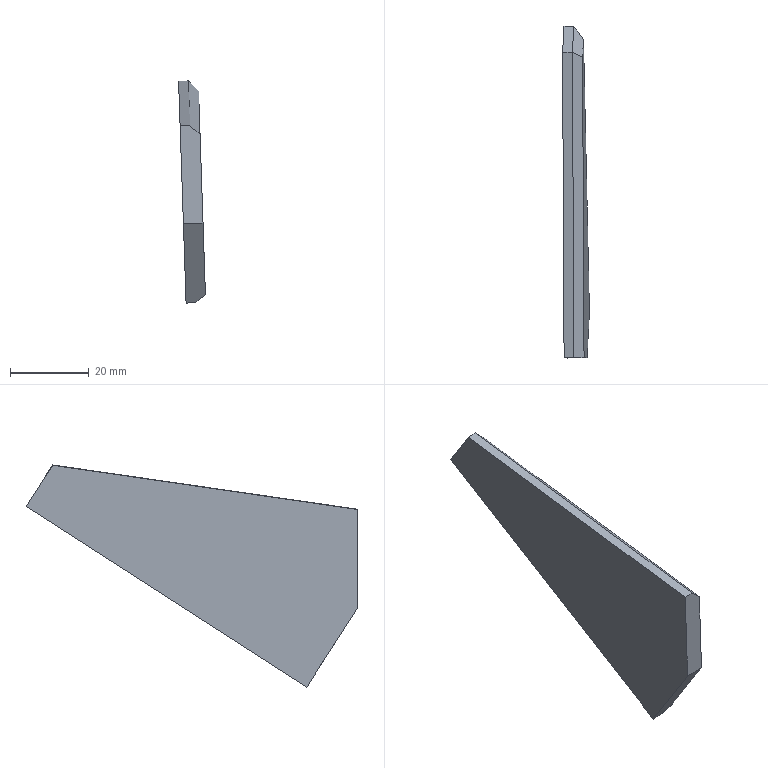Part | STEP file | 2026.6.15-Main Assembly图.sldasm-Part-153 | 1 solid | 10 faces | box 6.837 x 84.5 x 56.57 mm | volume 12087 mm3 | plane 10
STEP:
#1=CARTESIAN_POINT('',(-1629.423,663.579,4139.94));
#2=VERTEX_POINT('',#1);
#3=CARTESIAN_POINT('',(-1631.922,663.579,4139.856));
#4=VERTEX_POINT('',#3);
#5=CARTESIAN_POINT('',(-1626.925,663.579,4140.025));
#6=DIRECTION('',(-0.9994,0.,-0.03381));
#7=VECTOR('',#6,1000.);
#8=LINE('',#5,#7);
#9=EDGE_CURVE('',#2,#4,#8,.T.);
#10=ORIENTED_EDGE('',*,*,#9,.F.);
#11=CARTESIAN_POINT('',(-1626.996,662.226,4142.126));
#12=VERTEX_POINT('',#11);
#13=CARTESIAN_POINT('',(-1626.996,662.226,4142.126));
#14=DIRECTION('',(0.6866,-0.3827,0.6181));
#15=VECTOR('',#14,1000.);
#16=LINE('',#13,#15);
#17=EDGE_CURVE('',#2,#12,#16,.T.);
#18=ORIENTED_EDGE('',*,*,#17,.T.);
#19=CARTESIAN_POINT('',(-1627.609,650.551,4160.252));
#20=VERTEX_POINT('',#19);
#21=CARTESIAN_POINT('',(-1627.609,650.551,4160.252));
#22=DIRECTION('',(0.02843,0.5413,-0.8404));
#23=VECTOR('',#22,1000.);
#24=LINE('',#21,#23);
#25=EDGE_CURVE('',#20,#12,#24,.T.);
#26=ORIENTED_EDGE('',*,*,#25,.F.);
#27=CARTESIAN_POINT('',(-1632.606,650.551,4160.083));
#28=VERTEX_POINT('',#27);
#29=CARTESIAN_POINT('',(-1627.609,650.551,4160.252));
#30=DIRECTION('',(-0.9994,0.,-0.03381));
#31=VECTOR('',#30,1000.);
#32=LINE('',#29,#31);
#33=EDGE_CURVE('',#20,#28,#32,.T.);
#34=ORIENTED_EDGE('',*,*,#33,.T.);
#35=CARTESIAN_POINT('',(-1632.606,650.551,4160.083));
#36=DIRECTION('',(0.02843,0.5413,-0.8404));
#37=VECTOR('',#36,1000.);
#38=LINE('',#35,#37);
#39=EDGE_CURVE('',#28,#4,#38,.T.);
#40=ORIENTED_EDGE('',*,*,#39,.T.);
#41=EDGE_LOOP('',(#10,#18,#26,#34,#40));
#42=FACE_OUTER_BOUND('',#41,.T.);
#43=CARTESIAN_POINT('',(-1627.609,650.551,4160.252));
#44=DIRECTION('',(-0.0183,0.8409,0.541));
#45=DIRECTION('',(0.,-0.541,0.841));
#46=AXIS2_PLACEMENT_3D('',#43,#44,#45);
#47=PLANE('',#46);
#48=ADVANCED_FACE('',(#42),#47,.F.);
#49=CARTESIAN_POINT('',(-1630.979,735.051,4185.922));
#50=VERTEX_POINT('',#49);
#51=CARTESIAN_POINT('',(-1633.478,735.051,4185.837));
#52=VERTEX_POINT('',#51);
#53=CARTESIAN_POINT('',(-1628.481,735.051,4186.006));
#54=DIRECTION('',(-0.9994,0.,-0.03381));
#55=VECTOR('',#54,1000.);
#56=LINE('',#53,#55);
#57=EDGE_CURVE('',#50,#52,#56,.T.);
#58=ORIENTED_EDGE('',*,*,#57,.F.);
#59=CARTESIAN_POINT('',(-1629.423,663.579,4139.94));
#60=DIRECTION('',(0.0183,-0.8409,-0.541));
#61=VECTOR('',#60,1000.);
#62=LINE('',#59,#61);
#63=EDGE_CURVE('',#50,#2,#62,.T.);
#64=ORIENTED_EDGE('',*,*,#63,.T.);
#65=ORIENTED_EDGE('',*,*,#9,.T.);
#66=CARTESIAN_POINT('',(-1631.922,663.579,4139.856));
#67=DIRECTION('',(-0.0183,0.8409,0.541));
#68=VECTOR('',#67,1000.);
#69=LINE('',#66,#68);
#70=EDGE_CURVE('',#4,#52,#69,.T.);
#71=ORIENTED_EDGE('',*,*,#70,.T.);
#72=EDGE_LOOP('',(#58,#64,#65,#71));
#73=FACE_OUTER_BOUND('',#72,.T.);
#74=CARTESIAN_POINT('',(-1626.925,663.579,4140.025));
#75=DIRECTION('',(-0.02843,-0.5413,0.8404));
#76=DIRECTION('',(0.,-0.8407,-0.5415));
#77=AXIS2_PLACEMENT_3D('',#74,#75,#76);
#78=PLANE('',#77);
#79=ADVANCED_FACE('',(#73),#78,.F.);
#80=CARTESIAN_POINT('',(-1631.335,728.286,4196.426));
#81=VERTEX_POINT('',#80);
#82=CARTESIAN_POINT('',(-1633.833,728.286,4196.342));
#83=VERTEX_POINT('',#82);
#84=CARTESIAN_POINT('',(-1628.836,728.286,4196.511));
#85=DIRECTION('',(-0.9994,0.,-0.03381));
#86=VECTOR('',#85,1000.);
#87=LINE('',#84,#86);
#88=EDGE_CURVE('',#81,#83,#87,.T.);
#89=ORIENTED_EDGE('',*,*,#88,.F.);
#90=CARTESIAN_POINT('',(-1630.979,735.051,4185.922));
#91=DIRECTION('',(0.02843,0.5413,-0.8404));
#92=VECTOR('',#91,1000.);
#93=LINE('',#90,#92);
#94=EDGE_CURVE('',#81,#50,#93,.T.);
#95=ORIENTED_EDGE('',*,*,#94,.T.);
#96=ORIENTED_EDGE('',*,*,#57,.T.);
#97=CARTESIAN_POINT('',(-1633.478,735.051,4185.837));
#98=DIRECTION('',(-0.02843,-0.5413,0.8404));
#99=VECTOR('',#98,1000.);
#100=LINE('',#97,#99);
#101=EDGE_CURVE('',#52,#83,#100,.T.);
#102=ORIENTED_EDGE('',*,*,#101,.T.);
#103=EDGE_LOOP('',(#89,#95,#96,#102));
#104=FACE_OUTER_BOUND('',#103,.T.);
#105=CARTESIAN_POINT('',(-1628.481,735.051,4186.006));
#106=DIRECTION('',(0.0183,-0.8409,-0.541));
#107=DIRECTION('',(0.,0.541,-0.841));
#108=AXIS2_PLACEMENT_3D('',#105,#106,#107);
#109=PLANE('',#108);
#110=ADVANCED_FACE('',(#104),#109,.F.);
#111=CARTESIAN_POINT('',(-1630.953,650.551,4185.153));
#112=VERTEX_POINT('',#111);
#113=CARTESIAN_POINT('',(-1633.452,650.551,4185.069));
#114=VERTEX_POINT('',#113);
#115=CARTESIAN_POINT('',(-1628.455,650.551,4185.238));
#116=DIRECTION('',(-0.9994,0.,-0.03381));
#117=VECTOR('',#116,1000.);
#118=LINE('',#115,#117);
#119=EDGE_CURVE('',#112,#114,#118,.T.);
#120=ORIENTED_EDGE('',*,*,#119,.F.);
#121=CARTESIAN_POINT('',(-1631.335,728.286,4196.426));
#122=DIRECTION('',(-0.004856,0.9896,0.1435));
#123=VECTOR('',#122,1000.);
#124=LINE('',#121,#123);
#125=EDGE_CURVE('',#112,#81,#124,.T.);
#126=ORIENTED_EDGE('',*,*,#125,.T.);
#127=ORIENTED_EDGE('',*,*,#88,.T.);
#128=CARTESIAN_POINT('',(-1633.833,728.286,4196.342));
#129=DIRECTION('',(0.004856,-0.9896,-0.1435));
#130=VECTOR('',#129,1000.);
#131=LINE('',#128,#130);
#132=EDGE_CURVE('',#83,#114,#131,.T.);
#133=ORIENTED_EDGE('',*,*,#132,.T.);
#134=EDGE_LOOP('',(#120,#126,#127,#133));
#135=FACE_OUTER_BOUND('',#134,.T.);
#136=CARTESIAN_POINT('',(-1628.836,728.286,4196.511));
#137=DIRECTION('',(0.03346,0.1436,-0.9891));
#138=DIRECTION('',(0.,0.9896,0.1437));
#139=AXIS2_PLACEMENT_3D('',#136,#137,#138);
#140=PLANE('',#139);
#141=ADVANCED_FACE('',(#135),#140,.F.);
#142=CARTESIAN_POINT('',(-1628.369,650.551,4182.713));
#143=VERTEX_POINT('',#142);
#144=CARTESIAN_POINT('',(-1628.455,650.551,4185.238));
#145=DIRECTION('',(0.03381,0.,-0.9994));
#146=VECTOR('',#145,1000.);
#147=LINE('',#144,#146);
#148=EDGE_CURVE('',#143,#20,#147,.T.);
#149=ORIENTED_EDGE('',*,*,#148,.F.);
#150=CARTESIAN_POINT('',(-1610.613,650.551,4165.945));
#151=DIRECTION('',(-0.727,0.,0.6866));
#152=VECTOR('',#151,1000.);
#153=LINE('',#150,#152);
#154=EDGE_CURVE('',#143,#112,#153,.T.);
#155=ORIENTED_EDGE('',*,*,#154,.T.);
#156=ORIENTED_EDGE('',*,*,#119,.T.);
#157=CARTESIAN_POINT('',(-1633.452,650.551,4185.069));
#158=DIRECTION('',(0.03381,0.,-0.9994));
#159=VECTOR('',#158,1000.);
#160=LINE('',#157,#159);
#161=EDGE_CURVE('',#114,#28,#160,.T.);
#162=ORIENTED_EDGE('',*,*,#161,.T.);
#163=ORIENTED_EDGE('',*,*,#33,.F.);
#164=EDGE_LOOP('',(#149,#155,#156,#162,#163));
#165=FACE_OUTER_BOUND('',#164,.T.);
#166=CARTESIAN_POINT('',(-1628.455,650.551,4185.238));
#167=DIRECTION('',(0.,1.,0.));
#168=DIRECTION('',(-1.,0.,0.));
#169=AXIS2_PLACEMENT_3D('',#166,#167,#168);
#170=PLANE('',#169);
#171=ADVANCED_FACE('',(#165),#170,.F.);
#172=ORIENTED_EDGE('',*,*,#25,.T.);
#173=CARTESIAN_POINT('',(-1628.506,731.596,4186.755));
#174=VERTEX_POINT('',#173);
#175=CARTESIAN_POINT('',(-1628.552,733.698,4188.107));
#176=DIRECTION('',(-0.0183,0.8409,0.541));
#177=VECTOR('',#176,1000.);
#178=LINE('',#175,#177);
#179=EDGE_CURVE('',#12,#174,#178,.T.);
#180=ORIENTED_EDGE('',*,*,#179,.T.);
#181=CARTESIAN_POINT('',(-1628.745,727.054,4193.807));
#182=VERTEX_POINT('',#181);
#183=CARTESIAN_POINT('',(-1628.79,726.183,4195.158));
#184=DIRECTION('',(-0.02843,-0.5413,0.8404));
#185=VECTOR('',#184,1000.);
#186=LINE('',#183,#185);
#187=EDGE_CURVE('',#174,#182,#186,.T.);
#188=ORIENTED_EDGE('',*,*,#187,.T.);
#189=CARTESIAN_POINT('',(-1628.371,650.91,4182.765));
#190=DIRECTION('',(0.004856,-0.9896,-0.1435));
#191=VECTOR('',#190,1000.);
#192=LINE('',#189,#191);
#193=EDGE_CURVE('',#182,#143,#192,.T.);
#194=ORIENTED_EDGE('',*,*,#193,.T.);
#195=ORIENTED_EDGE('',*,*,#148,.T.);
#196=EDGE_LOOP('',(#172,#180,#188,#194,#195));
#197=FACE_OUTER_BOUND('',#196,.T.);
#198=CARTESIAN_POINT('',(-1628.954,406.261,4200.012));
#199=DIRECTION('',(0.9994,0.,0.03381));
#200=DIRECTION('',(0.03381,0.,-0.9994));
#201=AXIS2_PLACEMENT_3D('',#198,#199,#200);
#202=PLANE('',#201);
#203=ADVANCED_FACE('',(#197),#202,.T.);
#204=ORIENTED_EDGE('',*,*,#39,.F.);
#205=ORIENTED_EDGE('',*,*,#161,.F.);
#206=ORIENTED_EDGE('',*,*,#132,.F.);
#207=ORIENTED_EDGE('',*,*,#101,.F.);
#208=ORIENTED_EDGE('',*,*,#70,.F.);
#209=EDGE_LOOP('',(#204,#205,#206,#207,#208));
#210=FACE_OUTER_BOUND('',#209,.T.);
#211=CARTESIAN_POINT('',(-1633.952,406.261,4199.843));
#212=DIRECTION('',(0.9994,0.,0.03381));
#213=DIRECTION('',(0.03381,0.,-0.9994));
#214=AXIS2_PLACEMENT_3D('',#211,#212,#213);
#215=PLANE('',#214);
#216=ADVANCED_FACE('',(#210),#215,.F.);
#217=ORIENTED_EDGE('',*,*,#154,.F.);
#218=ORIENTED_EDGE('',*,*,#193,.F.);
#219=CARTESIAN_POINT('',(-1541.359,685.488,4105.449));
#220=DIRECTION('',(0.6669,-0.3172,-0.6743));
#221=VECTOR('',#220,1000.);
#222=LINE('',#219,#221);
#223=EDGE_CURVE('',#81,#182,#222,.T.);
#224=ORIENTED_EDGE('',*,*,#223,.F.);
#225=ORIENTED_EDGE('',*,*,#125,.F.);
#226=EDGE_LOOP('',(#217,#218,#224,#225));
#227=FACE_OUTER_BOUND('',#226,.T.);
#228=CARTESIAN_POINT('',(-1627.207,413.758,4148.373));
#229=DIRECTION('',(0.683,-0.1015,0.7233));
#230=DIRECTION('',(-0.004856,0.9896,0.1435));
#231=AXIS2_PLACEMENT_3D('',#228,#229,#230);
#232=PLANE('',#231);
#233=ADVANCED_FACE('',(#227),#232,.T.);
#234=ORIENTED_EDGE('',*,*,#223,.T.);
#235=ORIENTED_EDGE('',*,*,#187,.F.);
#236=CARTESIAN_POINT('',(-1566.758,645.33,4207.553));
#237=DIRECTION('',(0.5712,-0.798,0.1924));
#238=VECTOR('',#237,1000.);
#239=LINE('',#236,#238);
#240=EDGE_CURVE('',#50,#174,#239,.T.);
#241=ORIENTED_EDGE('',*,*,#240,.F.);
#242=ORIENTED_EDGE('',*,*,#94,.F.);
#243=EDGE_LOOP('',(#234,#235,#241,#242));
#244=FACE_OUTER_BOUND('',#243,.T.);
#245=CARTESIAN_POINT('',(-1633.83,630.246,4344.112));
#246=DIRECTION('',(0.6938,0.5946,0.4064));
#247=DIRECTION('',(0.02843,0.5413,-0.8404));
#248=AXIS2_PLACEMENT_3D('',#245,#246,#247);
#249=PLANE('',#248);
#250=ADVANCED_FACE('',(#244),#249,.T.);
#251=ORIENTED_EDGE('',*,*,#17,.F.);
#252=ORIENTED_EDGE('',*,*,#63,.F.);
#253=ORIENTED_EDGE('',*,*,#240,.T.);
#254=ORIENTED_EDGE('',*,*,#179,.F.);
#255=EDGE_LOOP('',(#251,#252,#253,#254));
#256=FACE_OUTER_BOUND('',#255,.T.);
#257=CARTESIAN_POINT('',(-1623.631,507.611,4042.655));
#258=DIRECTION('',(0.7268,0.3827,-0.5703));
#259=DIRECTION('',(0.0183,-0.8409,-0.541));
#260=AXIS2_PLACEMENT_3D('',#257,#258,#259);
#261=PLANE('',#260);
#262=ADVANCED_FACE('',(#256),#261,.T.);
#263=CLOSED_SHELL('',(#48,#79,#110,#141,#171,#203,#216,#233,#250,#262));
#264=MANIFOLD_SOLID_BREP('',#263);
#265=CARTESIAN_POINT('',(0.,0.,0.));
#266=DIRECTION('',(0.,0.,1.));
#267=DIRECTION('',(1.,0.,0.));
#268=AXIS2_PLACEMENT_3D('',#265,#266,#267);
#269=(LENGTH_UNIT()NAMED_UNIT(*)SI_UNIT(.MILLI.,.METRE.));
#270=UNCERTAINTY_MEASURE_WITH_UNIT(LENGTH_MEASURE(0.00001),#269,'','');
#271=(NAMED_UNIT(*)PLANE_ANGLE_UNIT()SI_UNIT($,.RADIAN.));
#272=(NAMED_UNIT(*)SI_UNIT($,.STERADIAN.)SOLID_ANGLE_UNIT());
#273=(GEOMETRIC_REPRESENTATION_CONTEXT(3)GLOBAL_UNCERTAINTY_ASSIGNED_CONTEXT((#270))GLOBAL_UNIT_ASSIGNED_CONTEXT((#269,#271,#272))REPRESENTATION_CONTEXT('',''));
#274=ADVANCED_BREP_SHAPE_REPRESENTATION('',(#264,#268),#273);